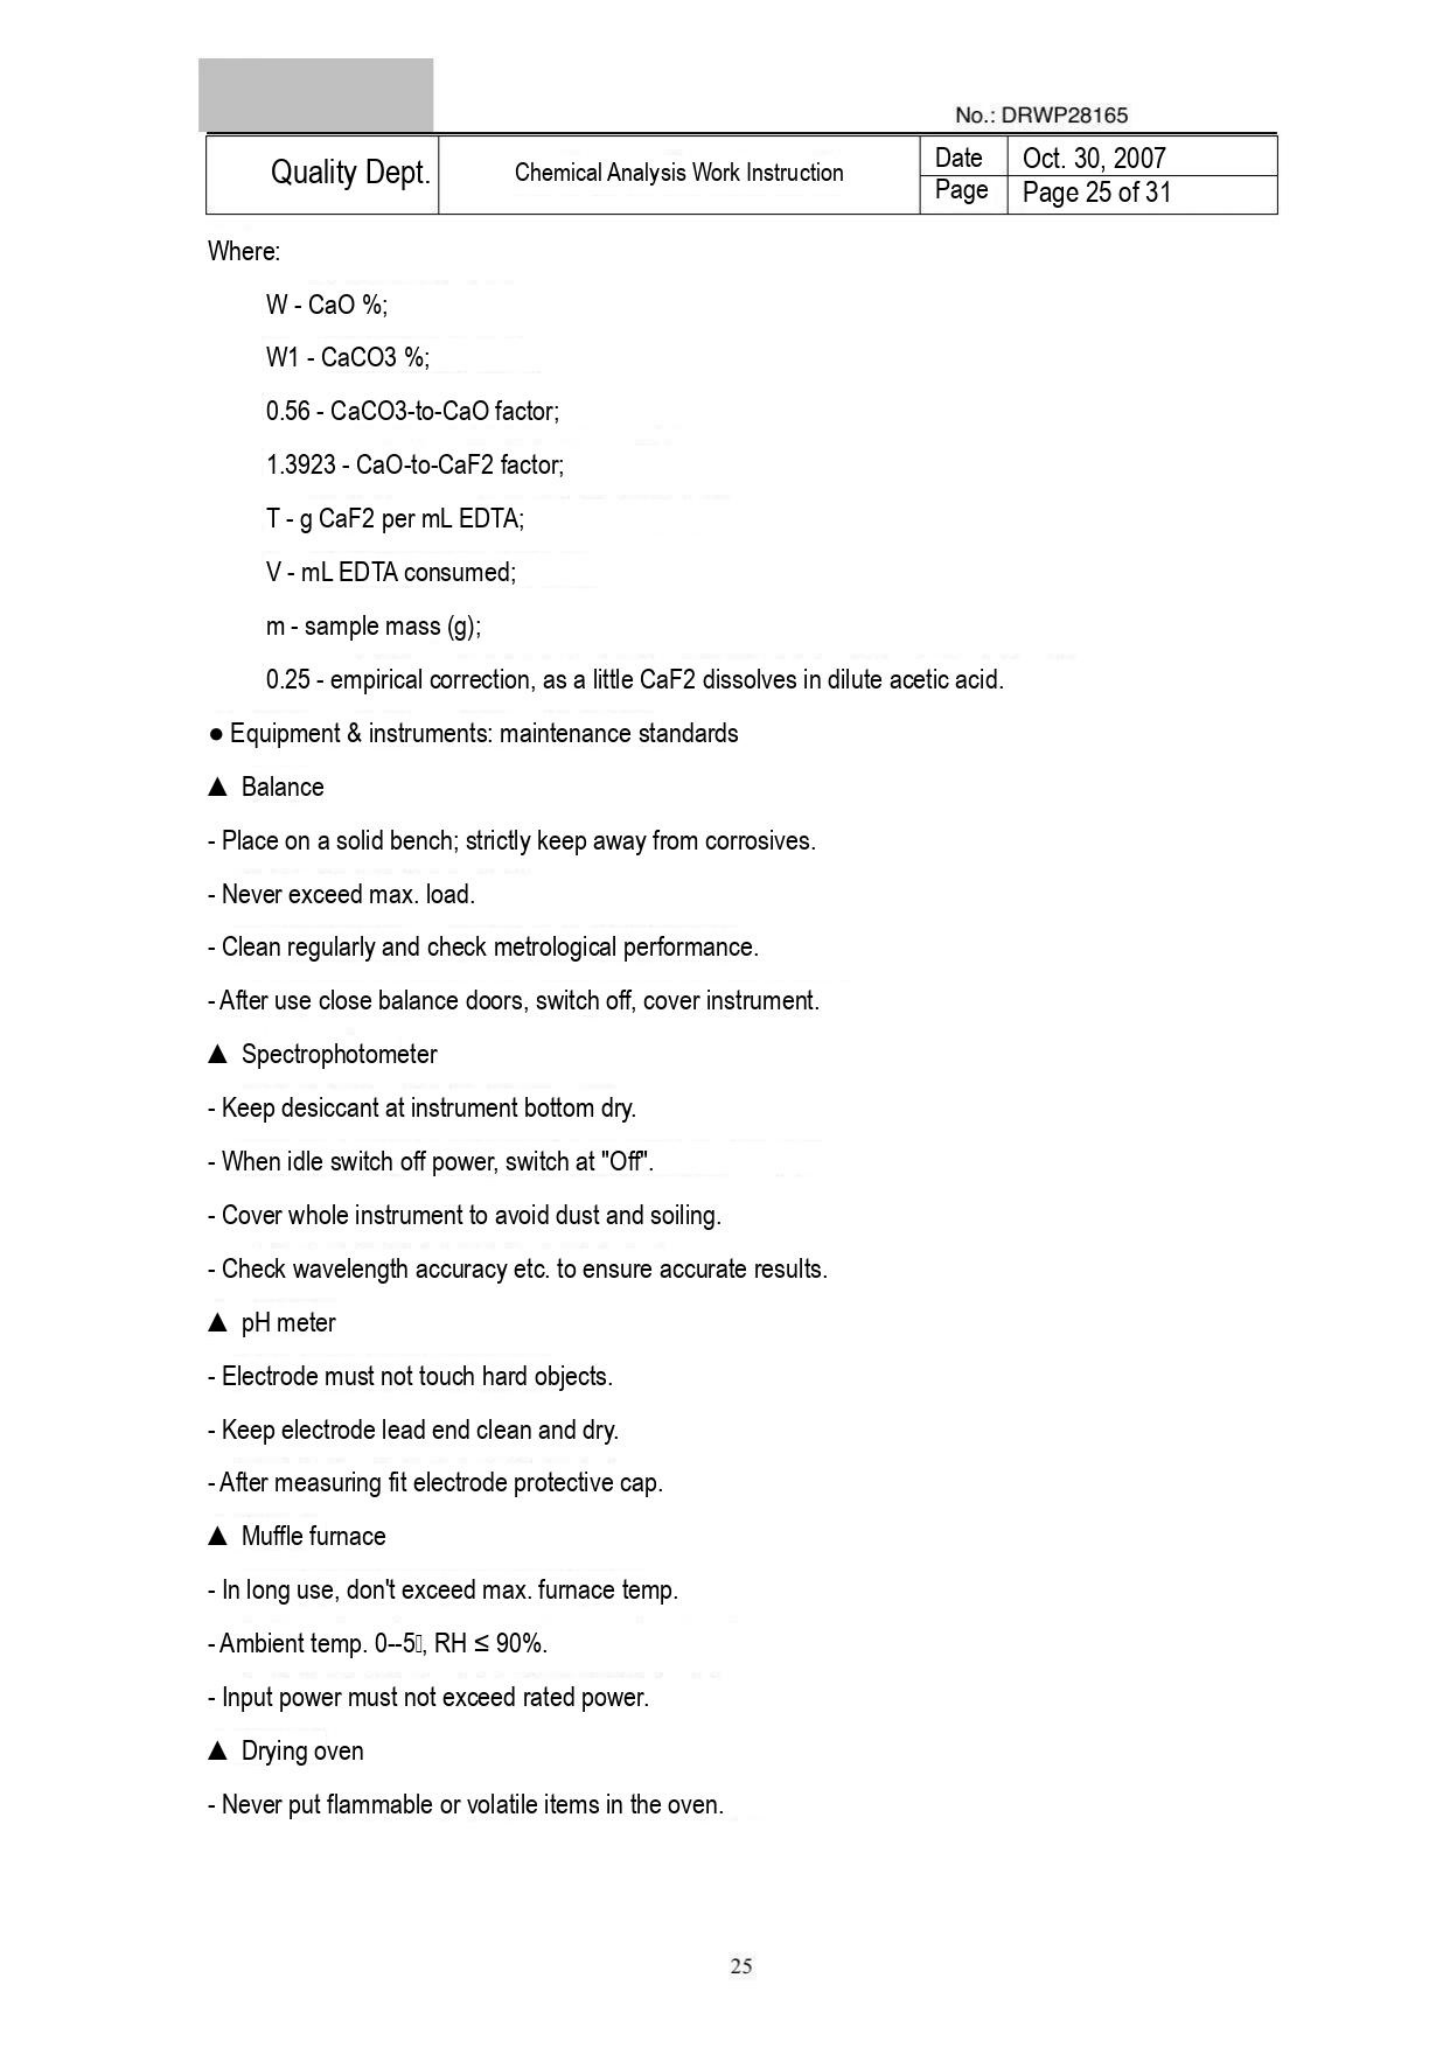No.: DRWP28165

| Quality Dept. | Chemical Analysis Work Instruction | Date | Oct. 30, 2007 |
|---|---|---|---|
| | | Page | Page 25 of 31 |

Where:

W - CaO %;

W1 - CaCO3 %;

0.56 - CaCO3-to-CaO factor;

1.3923 - CaO-to-CaF2 factor;

T - g CaF2 per mL EDTA;

V - mL EDTA consumed;

m - sample mass (g);

0.25 - empirical correction, as a little CaF2 dissolves in dilute acetic acid.

● Equipment & instruments: maintenance standards

▲ Balance

- Place on a solid bench; strictly keep away from corrosives.

- Never exceed max. load.

- Clean regularly and check metrological performance.

- After use close balance doors, switch off, cover instrument.

▲ Spectrophotometer

- Keep desiccant at instrument bottom dry.

- When idle switch off power, switch at "Off".

- Cover whole instrument to avoid dust and soiling.

- Check wavelength accuracy etc. to ensure accurate results.

▲ pH meter

- Electrode must not touch hard objects.

- Keep electrode lead end clean and dry.

- After measuring fit electrode protective cap.

▲ Muffle furnace

- In long use, don't exceed max. furnace temp.

- Ambient temp. 0--5, RH ≤ 90%.

- Input power must not exceed rated power.

▲ Drying oven

- Never put flammable or volatile items in the oven.

25
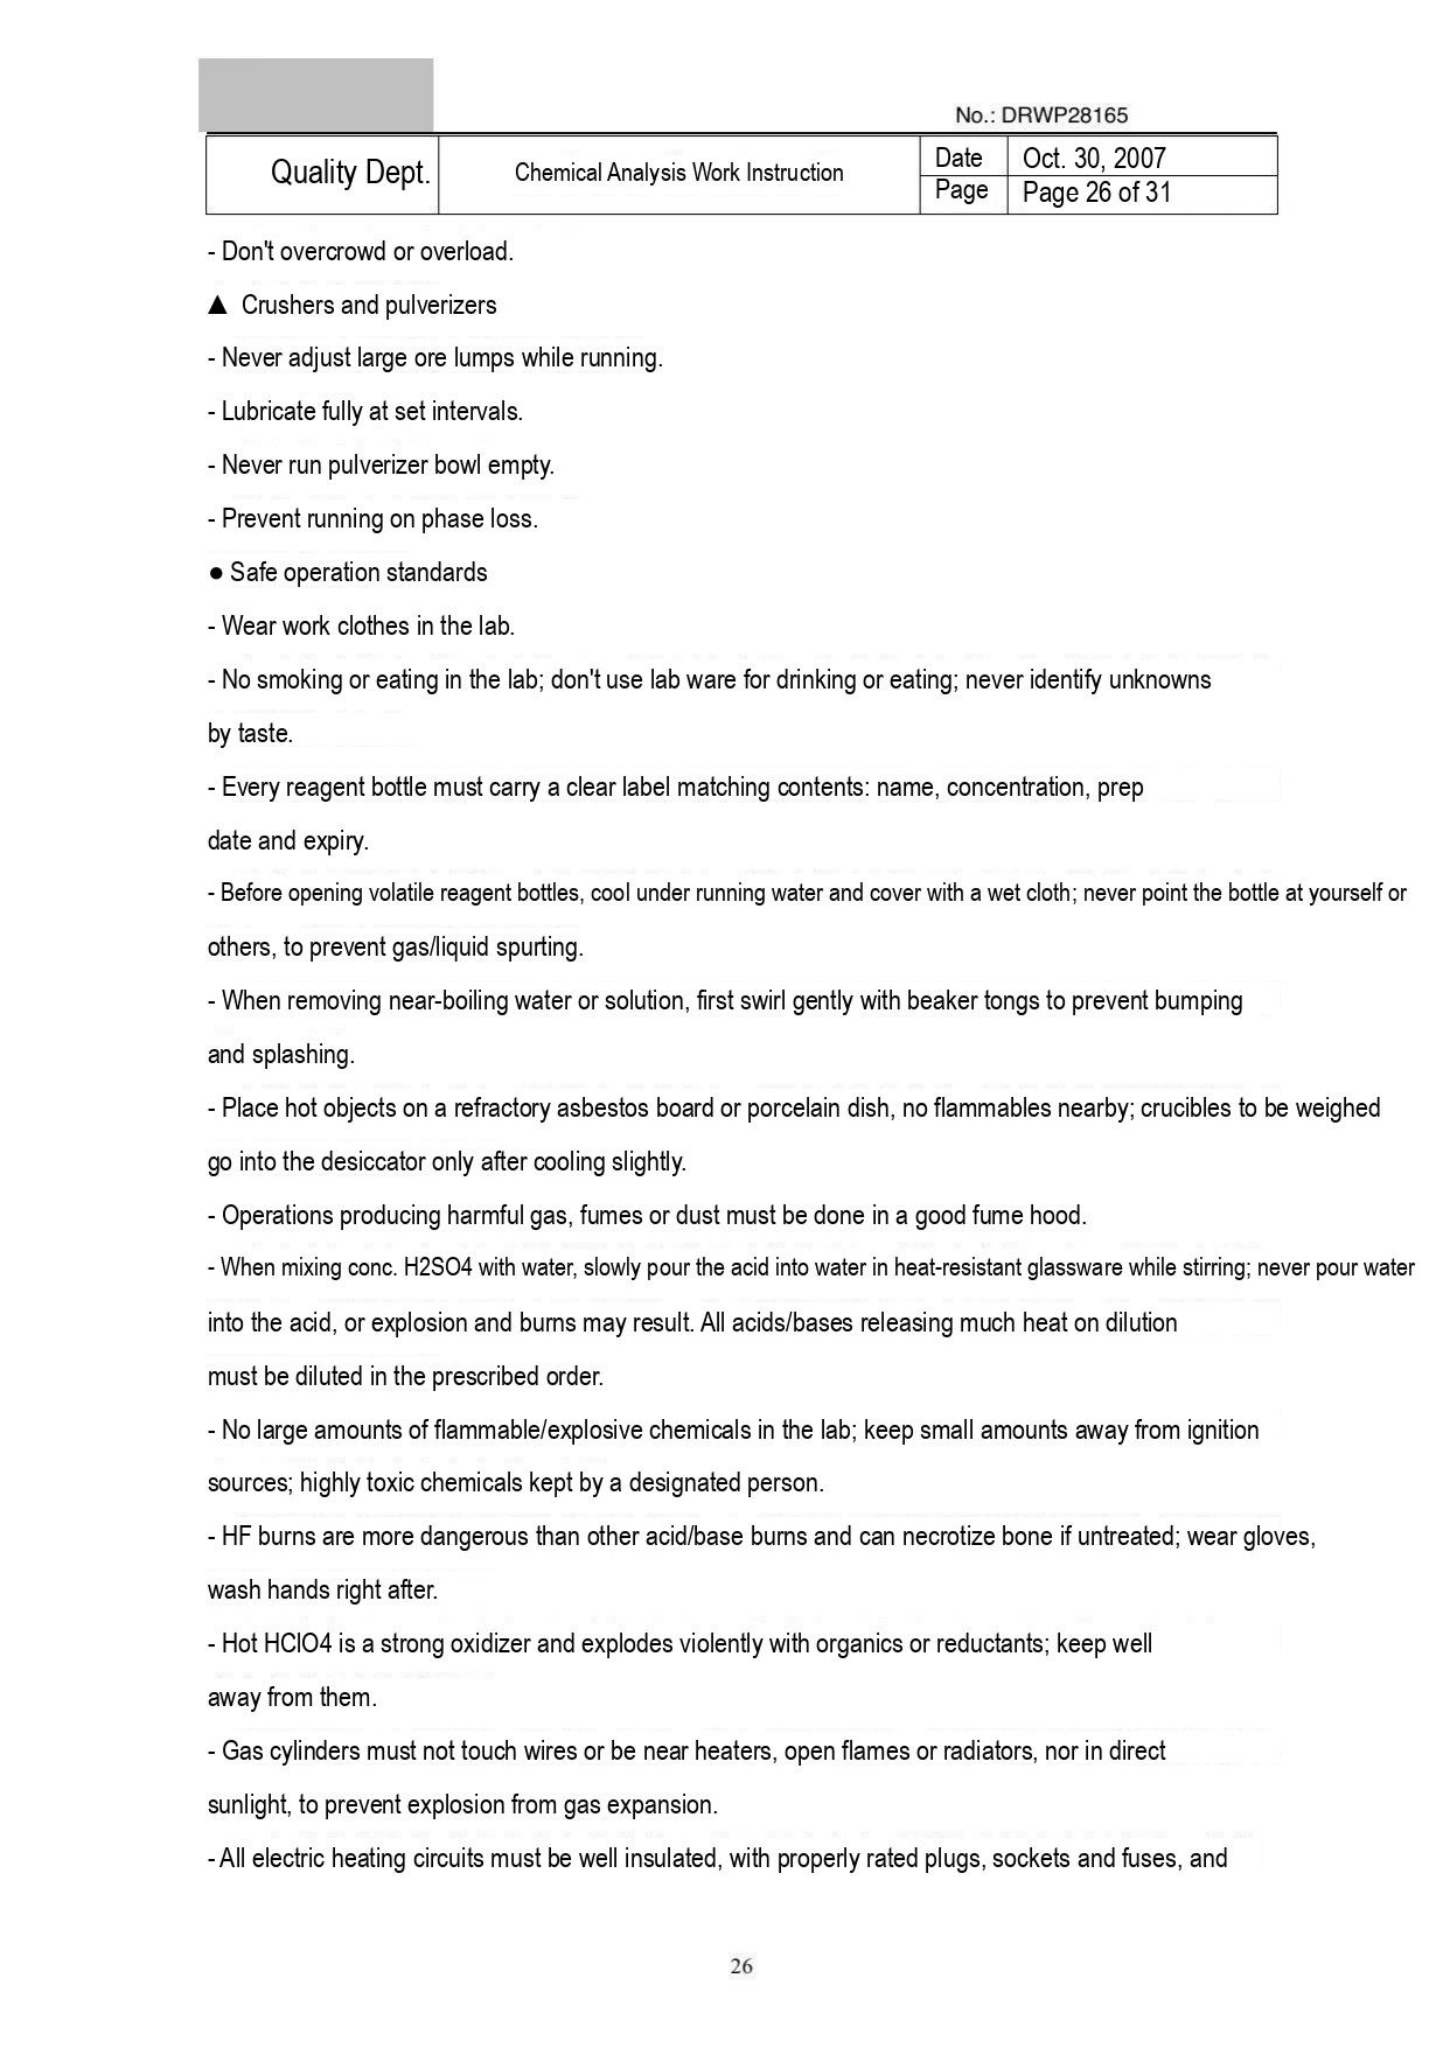No.: DRWP28165

| Quality Dept. | Chemical Analysis Work Instruction | Date | Oct. 30, 2007 |
|---|---|---|---|
| | | Page | Page 26 of 31 |

- Don't overcrowd or overload.

▲ Crushers and pulverizers

- Never adjust large ore lumps while running.

- Lubricate fully at set intervals.

- Never run pulverizer bowl empty.

- Prevent running on phase loss.

● Safe operation standards

- Wear work clothes in the lab.

- No smoking or eating in the lab; don't use lab ware for drinking or eating; never identify unknowns by taste.

- Every reagent bottle must carry a clear label matching contents: name, concentration, prep date and expiry.

- Before opening volatile reagent bottles, cool under running water and cover with a wet cloth; never point the bottle at yourself or others, to prevent gas/liquid spurting.

- When removing near-boiling water or solution, first swirl gently with beaker tongs to prevent bumping and splashing.

- Place hot objects on a refractory asbestos board or porcelain dish, no flammables nearby; crucibles to be weighed go into the desiccator only after cooling slightly.

- Operations producing harmful gas, fumes or dust must be done in a good fume hood.

- When mixing conc. H2SO4 with water, slowly pour the acid into water in heat-resistant glassware while stirring; never pour water into the acid, or explosion and burns may result. All acids/bases releasing much heat on dilution must be diluted in the prescribed order.

- No large amounts of flammable/explosive chemicals in the lab; keep small amounts away from ignition sources; highly toxic chemicals kept by a designated person.

- HF burns are more dangerous than other acid/base burns and can necrotize bone if untreated; wear gloves, wash hands right after.

- Hot HClO4 is a strong oxidizer and explodes violently with organics or reductants; keep well away from them.

- Gas cylinders must not touch wires or be near heaters, open flames or radiators, nor in direct sunlight, to prevent explosion from gas expansion.

- All electric heating circuits must be well insulated, with properly rated plugs, sockets and fuses, and

26
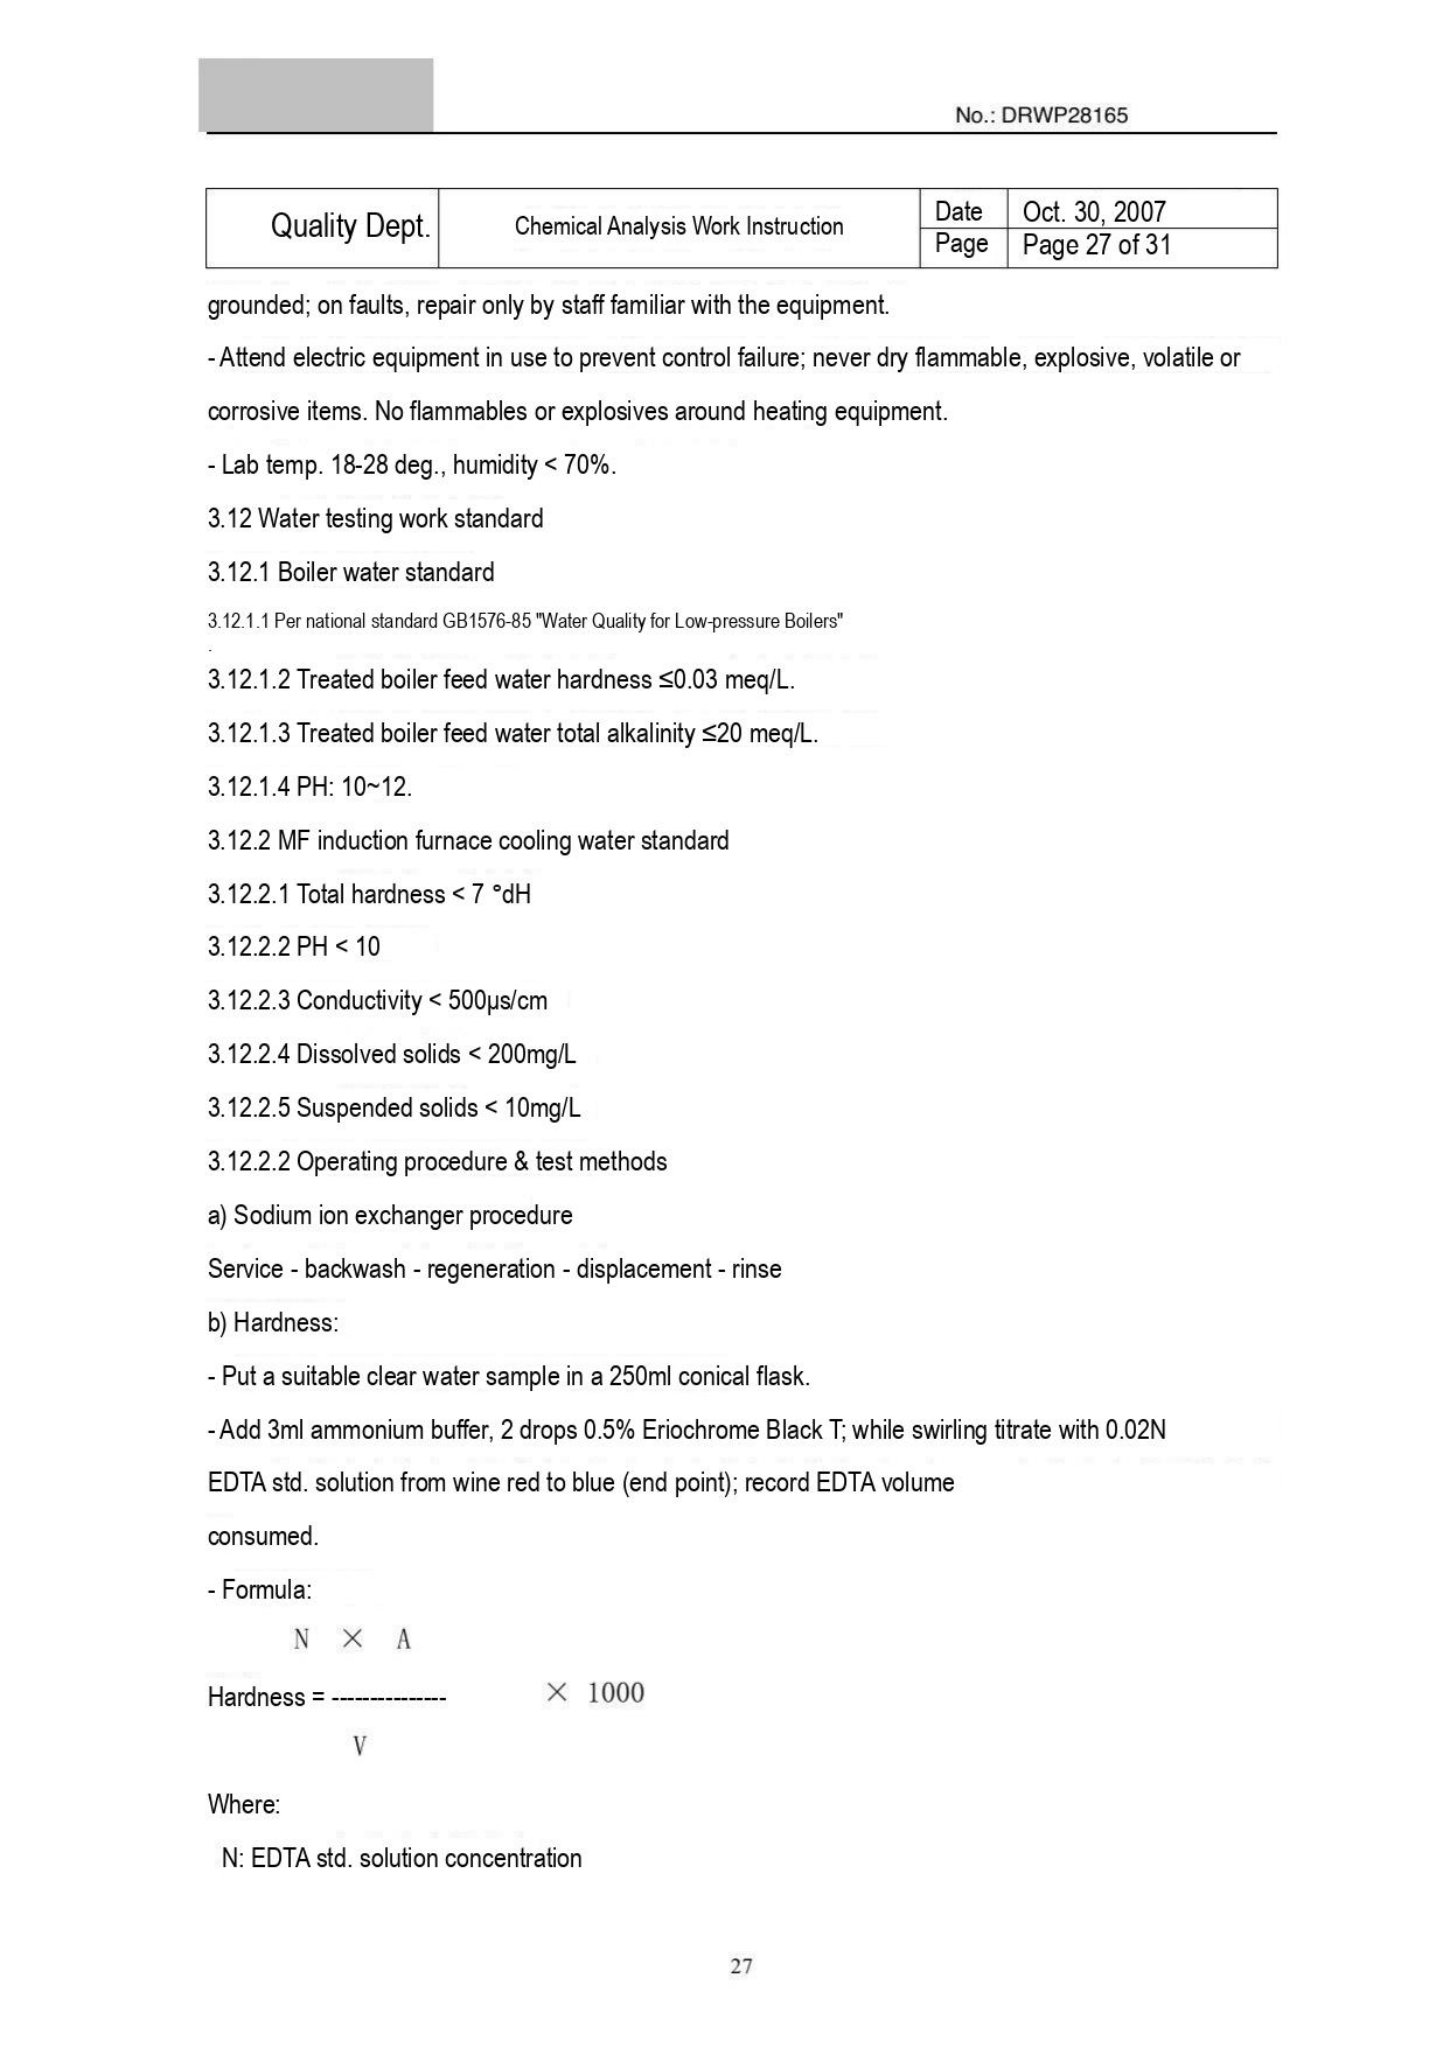No.: DRWP28165

| Quality Dept. | Chemical Analysis Work Instruction | Date | Oct. 30, 2007 |
|---|---|---|---|
| | | Page | Page 27 of 31 |

grounded; on faults, repair only by staff familiar with the equipment.

- Attend electric equipment in use to prevent control failure; never dry flammable, explosive, volatile or corrosive items. No flammables or explosives around heating equipment.

- Lab temp. 18-28 deg., humidity < 70%.

3.12 Water testing work standard

3.12.1 Boiler water standard

3.12.1.1 Per national standard GB1576-85 "Water Quality for Low-pressure Boilers"

3.12.1.2 Treated boiler feed water hardness ≤0.03 meq/L.

3.12.1.3 Treated boiler feed water total alkalinity ≤20 meq/L.

3.12.1.4 PH: 10~12.

3.12.2 MF induction furnace cooling water standard

3.12.2.1 Total hardness < 7 °dH

3.12.2.2 PH < 10

3.12.2.3 Conductivity < 500μs/cm

3.12.2.4 Dissolved solids < 200mg/L

3.12.2.5 Suspended solids < 10mg/L

3.12.2.2 Operating procedure & test methods

a) Sodium ion exchanger procedure

Service - backwash - regeneration - displacement - rinse

b) Hardness:

- Put a suitable clear water sample in a 250ml conical flask.

- Add 3ml ammonium buffer, 2 drops 0.5% Eriochrome Black T; while swirling titrate with 0.02N EDTA std. solution from wine red to blue (end point); record EDTA volume consumed.

- Formula:

N × A

Hardness = -------------- × 1000

V

Where:

N: EDTA std. solution concentration

27
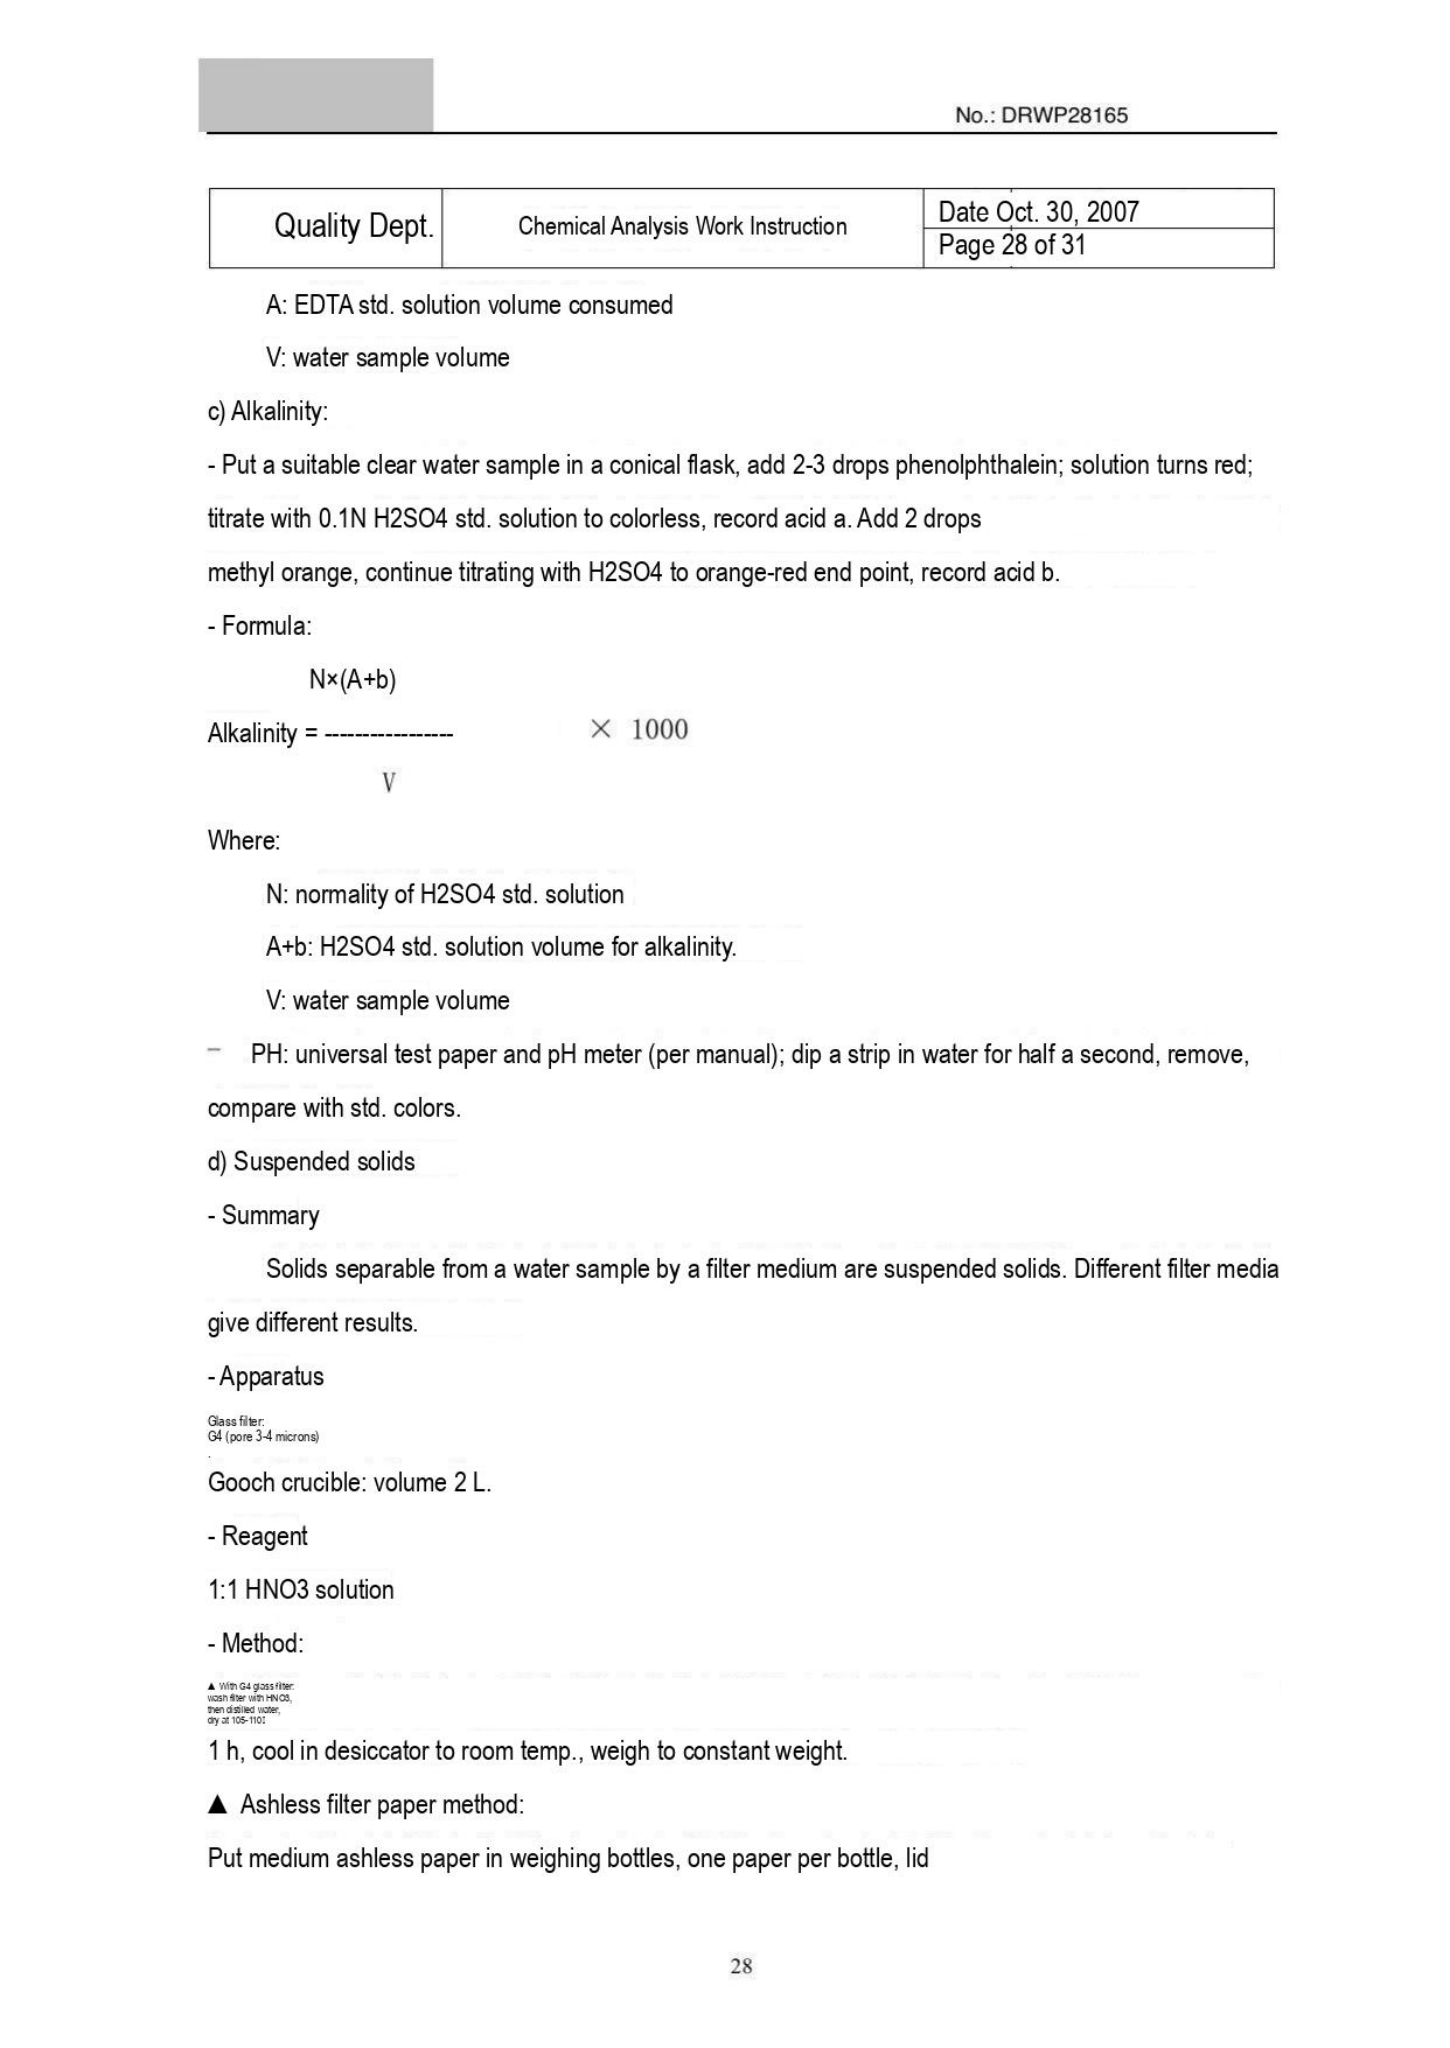No.: DRWP28165

| Quality Dept. | Chemical Analysis Work Instruction | Date Oct. 30, 2007<br>Page 28 of 31 |
|---|---|---|

A: EDTA std. solution volume consumed

V: water sample volume

c) Alkalinity:

- Put a suitable clear water sample in a conical flask, add 2-3 drops phenolphthalein; solution turns red; titrate with 0.1N H2SO4 std. solution to colorless, record acid a. Add 2 drops methyl orange, continue titrating with H2SO4 to orange-red end point, record acid b.

- Formula:

N×(A+b)

Alkalinity = ---------------- × 1000

V

Where:

N: normality of H2SO4 std. solution

A+b: H2SO4 std. solution volume for alkalinity.

V: water sample volume

– PH: universal test paper and pH meter (per manual); dip a strip in water for half a second, remove, compare with std. colors.

d) Suspended solids

- Summary

Solids separable from a water sample by a filter medium are suspended solids. Different filter media give different results.

- Apparatus

Glass filter:
G4 (pore 3-4 microns)

Gooch crucible: volume 2 L.

- Reagent

1:1 HNO3 solution

- Method:

▲ With G4 glass filter:
wash filter with HNO3,
then distilled water,
dry at 105-110

1 h, cool in desiccator to room temp., weigh to constant weight.

▲ Ashless filter paper method:

Put medium ashless paper in weighing bottles, one paper per bottle, lid

28
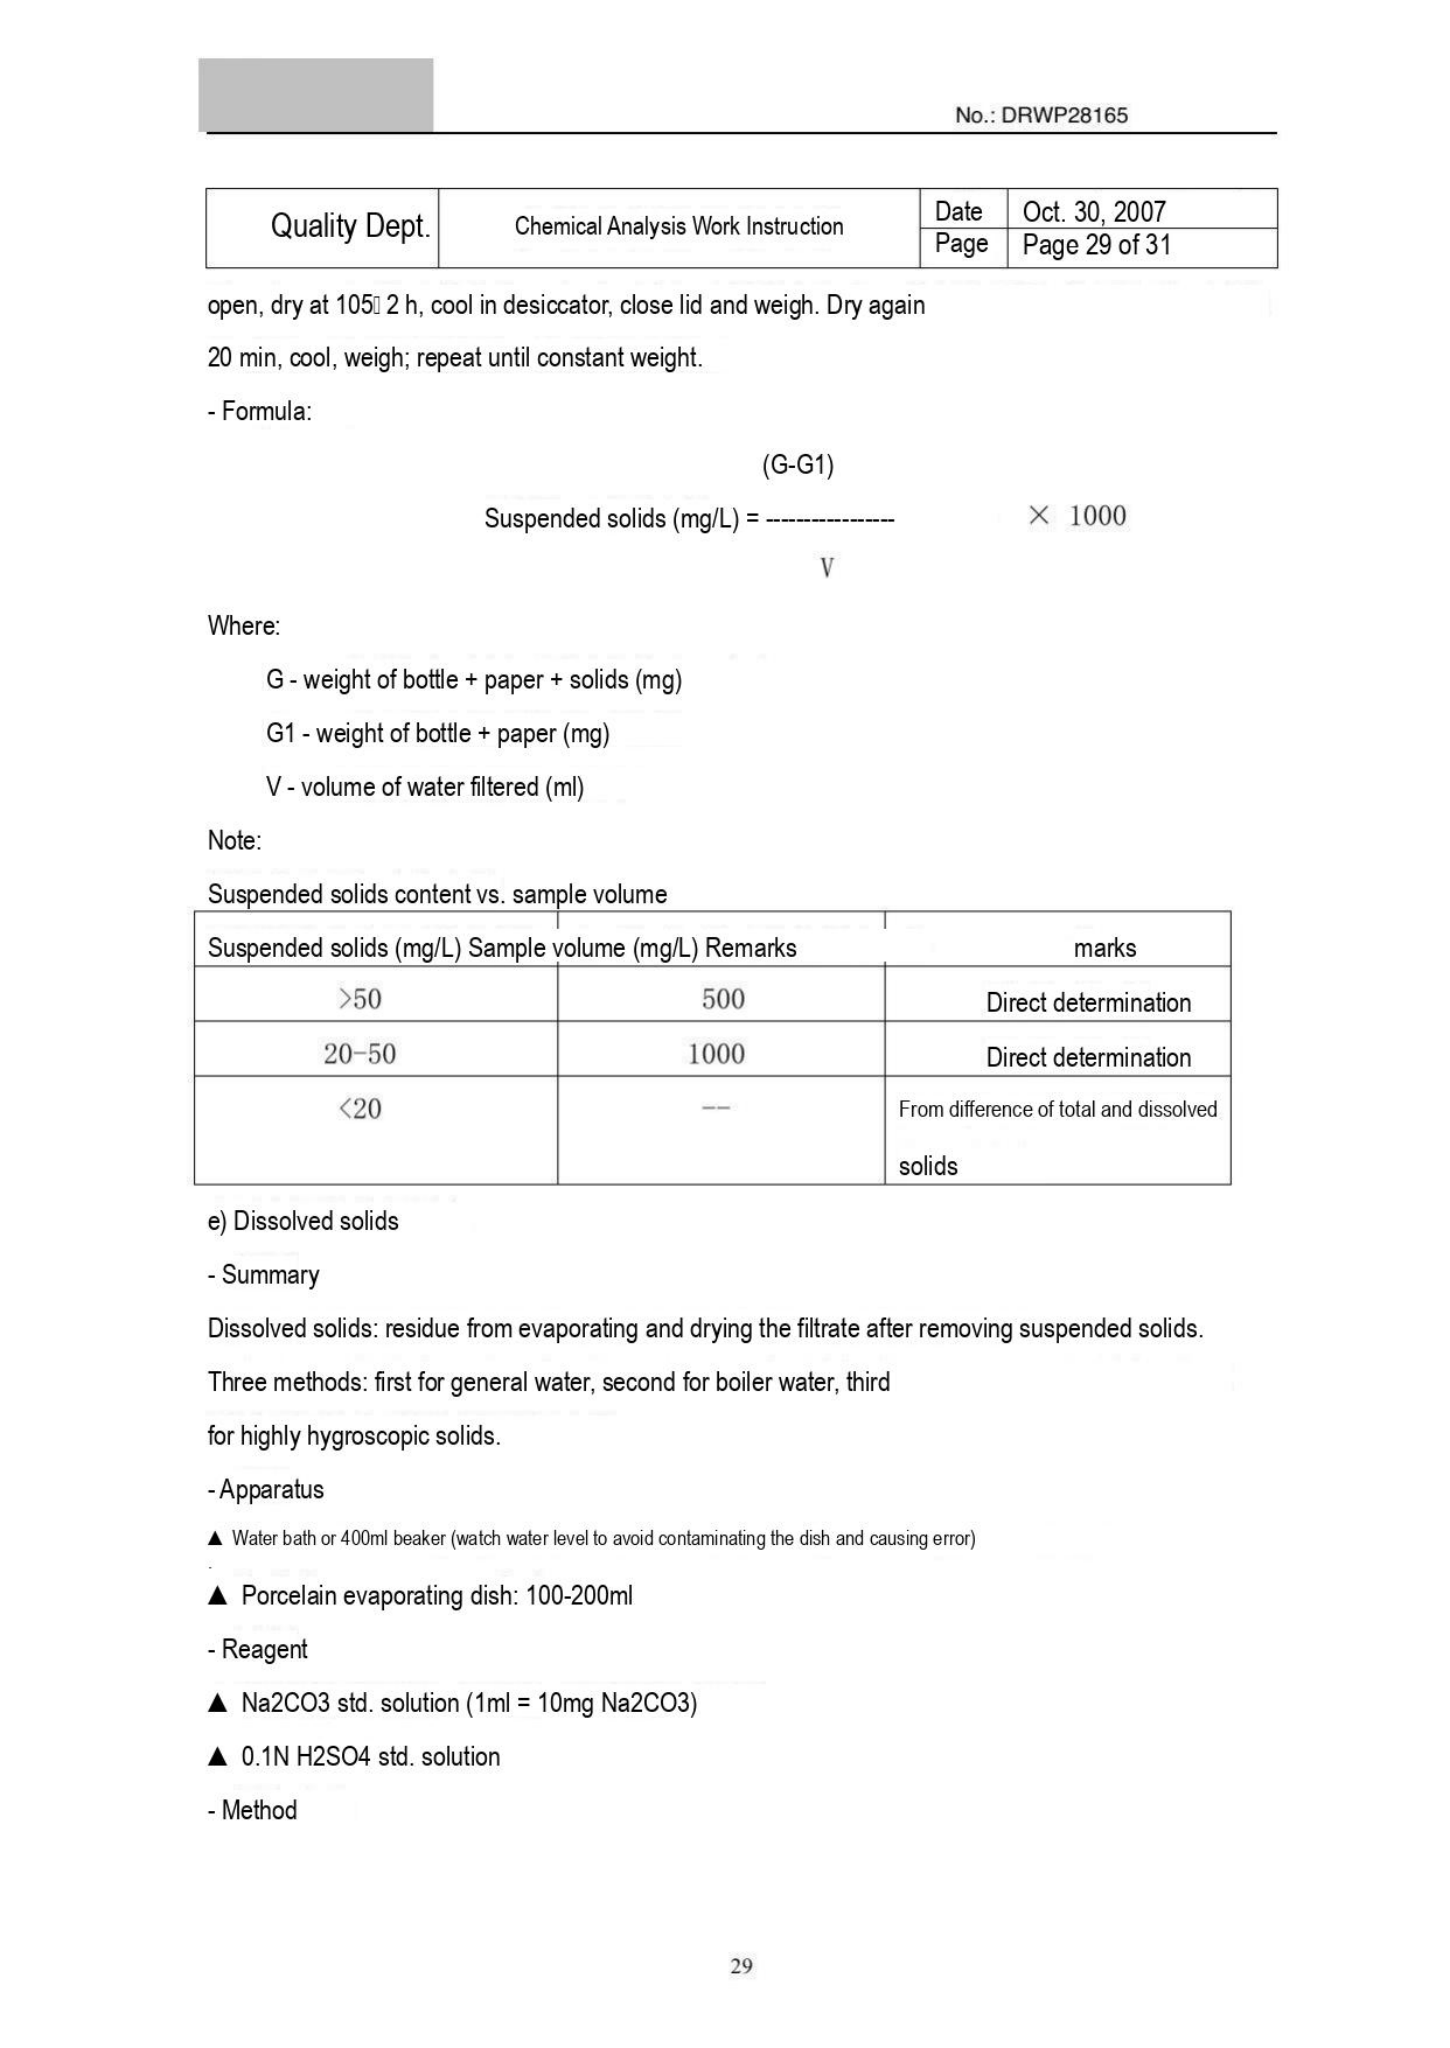No.: DRWP28165

| Quality Dept. | Chemical Analysis Work Instruction | Date | Oct. 30, 2007 |
|---|---|---|---|
| | | Page | Page 29 of 31 |

open, dry at 105 2 h, cool in desiccator, close lid and weigh. Dry again

20 min, cool, weigh; repeat until constant weight.

- Formula:

(G-G1)

Suspended solids (mg/L) = ---------------- × 1000

V

Where:

G - weight of bottle + paper + solids (mg)

G1 - weight of bottle + paper (mg)

V - volume of water filtered (ml)

Note:

Suspended solids content vs. sample volume

| Suspended solids (mg/L) Sample volume (mg/L) Remarks | | marks |
|---|---|---|
| >50 | 500 | Direct determination |
| 20−50 | 1000 | Direct determination |
| <20 | -- | From difference of total and dissolved solids |

e) Dissolved solids

- Summary

Dissolved solids: residue from evaporating and drying the filtrate after removing suspended solids.

Three methods: first for general water, second for boiler water, third

for highly hygroscopic solids.

- Apparatus

▲ Water bath or 400ml beaker (watch water level to avoid contaminating the dish and causing error)

▲ Porcelain evaporating dish: 100-200ml

- Reagent

▲ Na2CO3 std. solution (1ml = 10mg Na2CO3)

▲ 0.1N H2SO4 std. solution

- Method

29
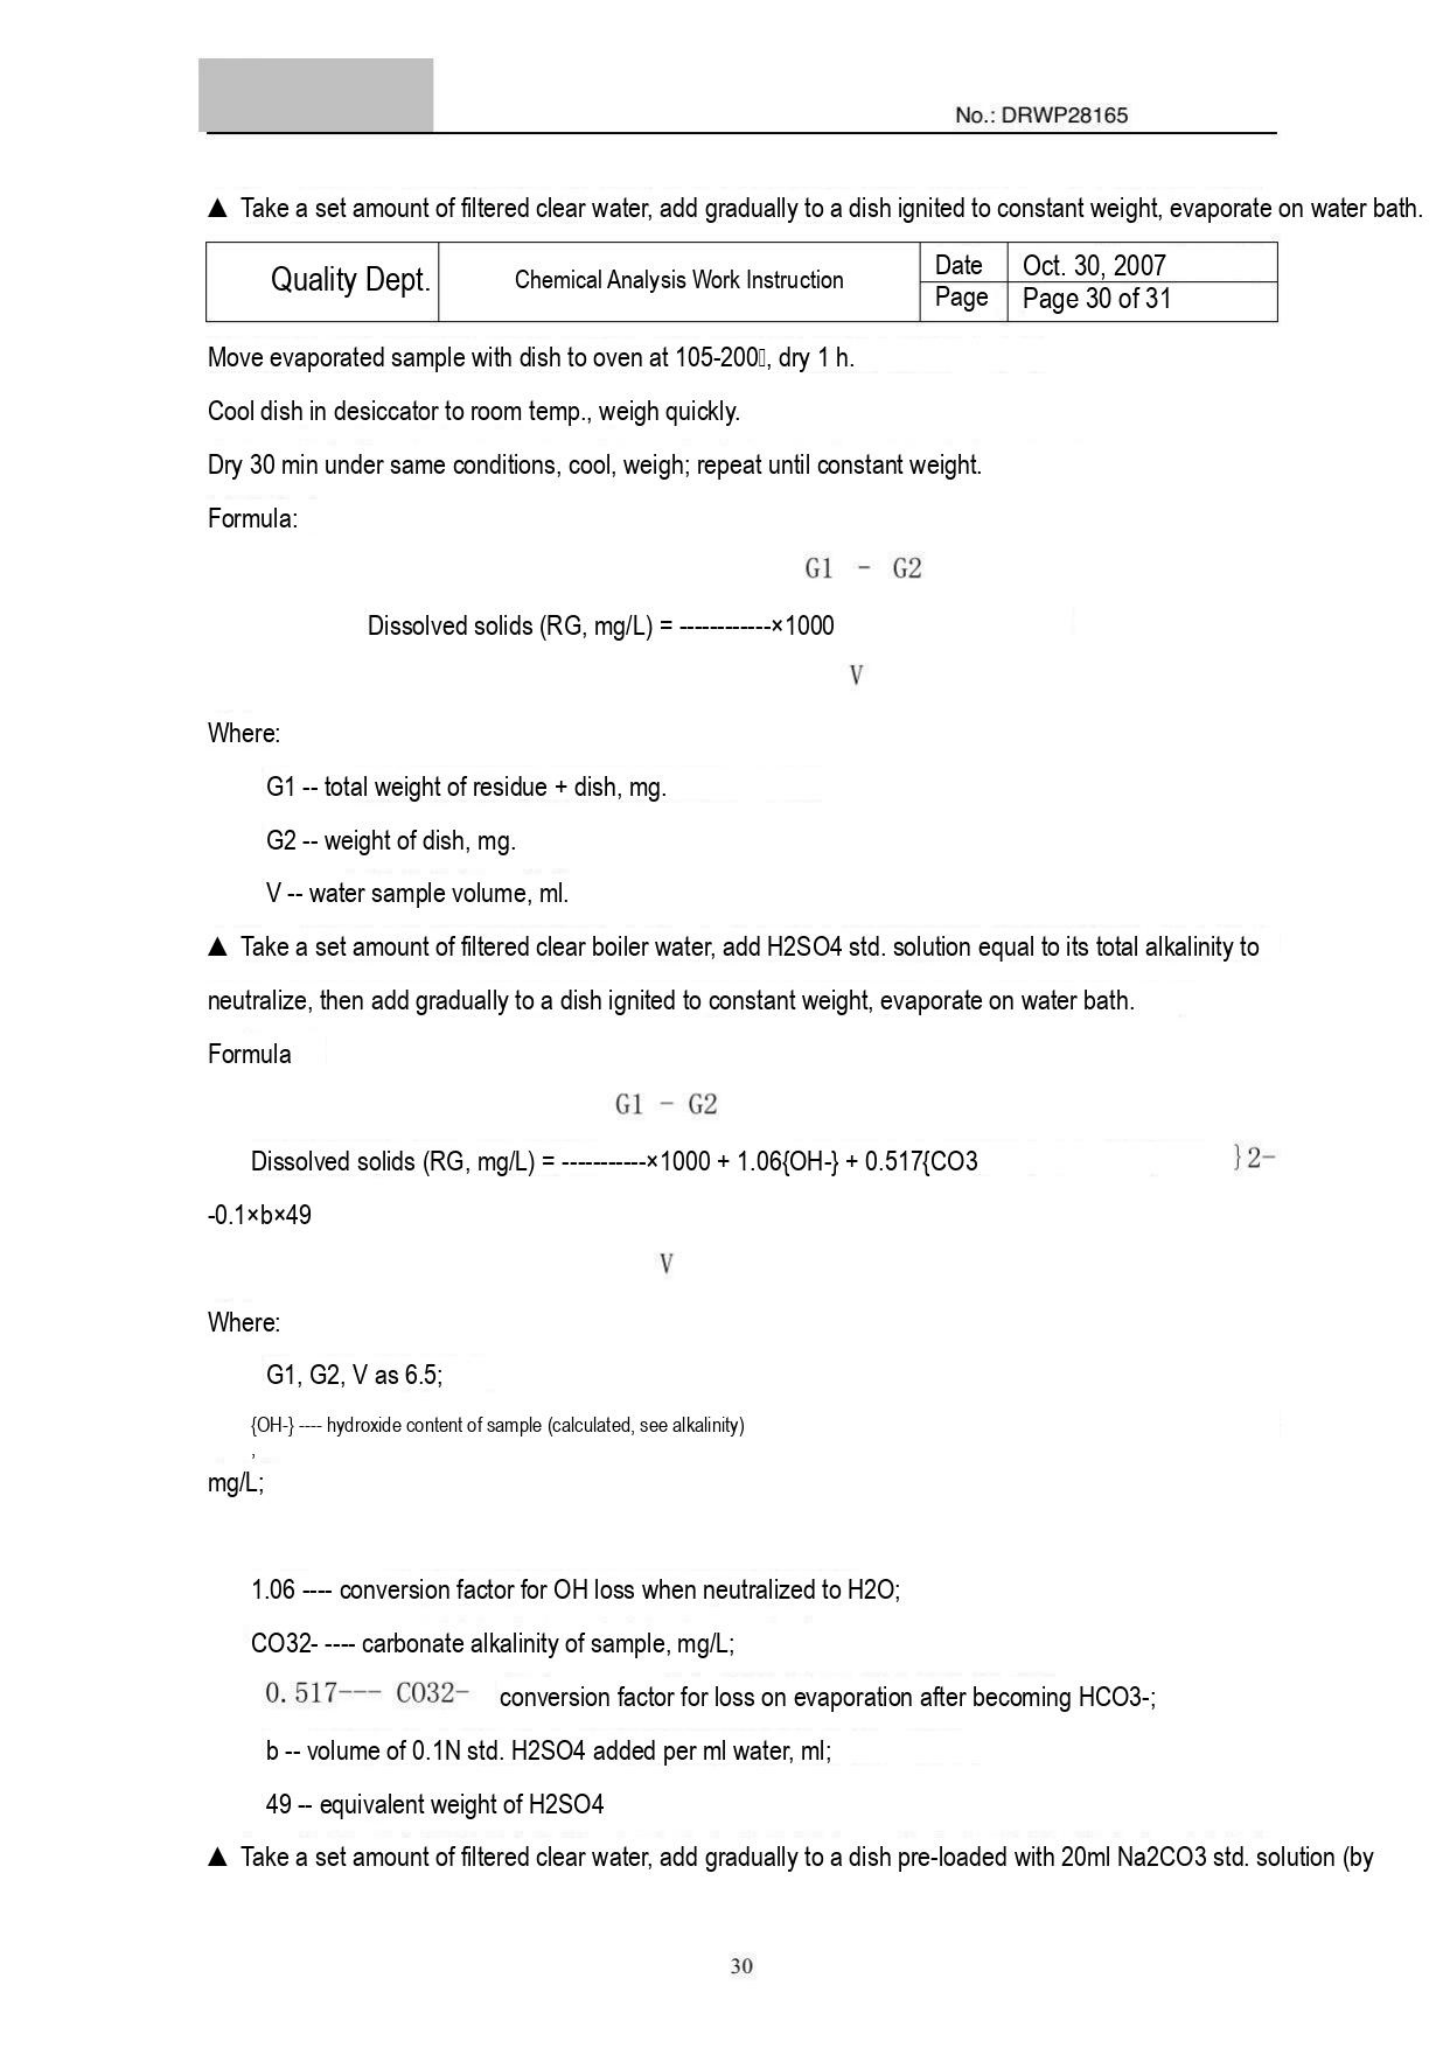No.: DRWP28165

▲ Take a set amount of filtered clear water, add gradually to a dish ignited to constant weight, evaporate on water bath.

| Quality Dept. | Chemical Analysis Work Instruction | Date | Oct. 30, 2007 |
|---|---|---|---|
| | | Page | Page 30 of 31 |

Move evaporated sample with dish to oven at 105-200, dry 1 h.

Cool dish in desiccator to room temp., weigh quickly.

Dry 30 min under same conditions, cool, weigh; repeat until constant weight.

Formula:

G1 - G2

Dissolved solids (RG, mg/L) = -----------×1000

V

Where:

G1 -- total weight of residue + dish, mg.

G2 -- weight of dish, mg.

V -- water sample volume, ml.

▲ Take a set amount of filtered clear boiler water, add H2SO4 std. solution equal to its total alkalinity to neutralize, then add gradually to a dish ignited to constant weight, evaporate on water bath.

Formula

G1 - G2

Dissolved solids (RG, mg/L) = ----------×1000 + 1.06{OH-} + 0.517{CO3 }2-

-0.1×b×49

V

Where:

G1, G2, V as 6.5;

{OH-} ---- hydroxide content of sample (calculated, see alkalinity)

,

mg/L;

1.06 ---- conversion factor for OH loss when neutralized to H2O;

CO32- ---- carbonate alkalinity of sample, mg/L;

0.517--- CO32- conversion factor for loss on evaporation after becoming HCO3-;

b -- volume of 0.1N std. H2SO4 added per ml water, ml;

49 -- equivalent weight of H2SO4

▲ Take a set amount of filtered clear water, add gradually to a dish pre-loaded with 20ml Na2CO3 std. solution (by

30
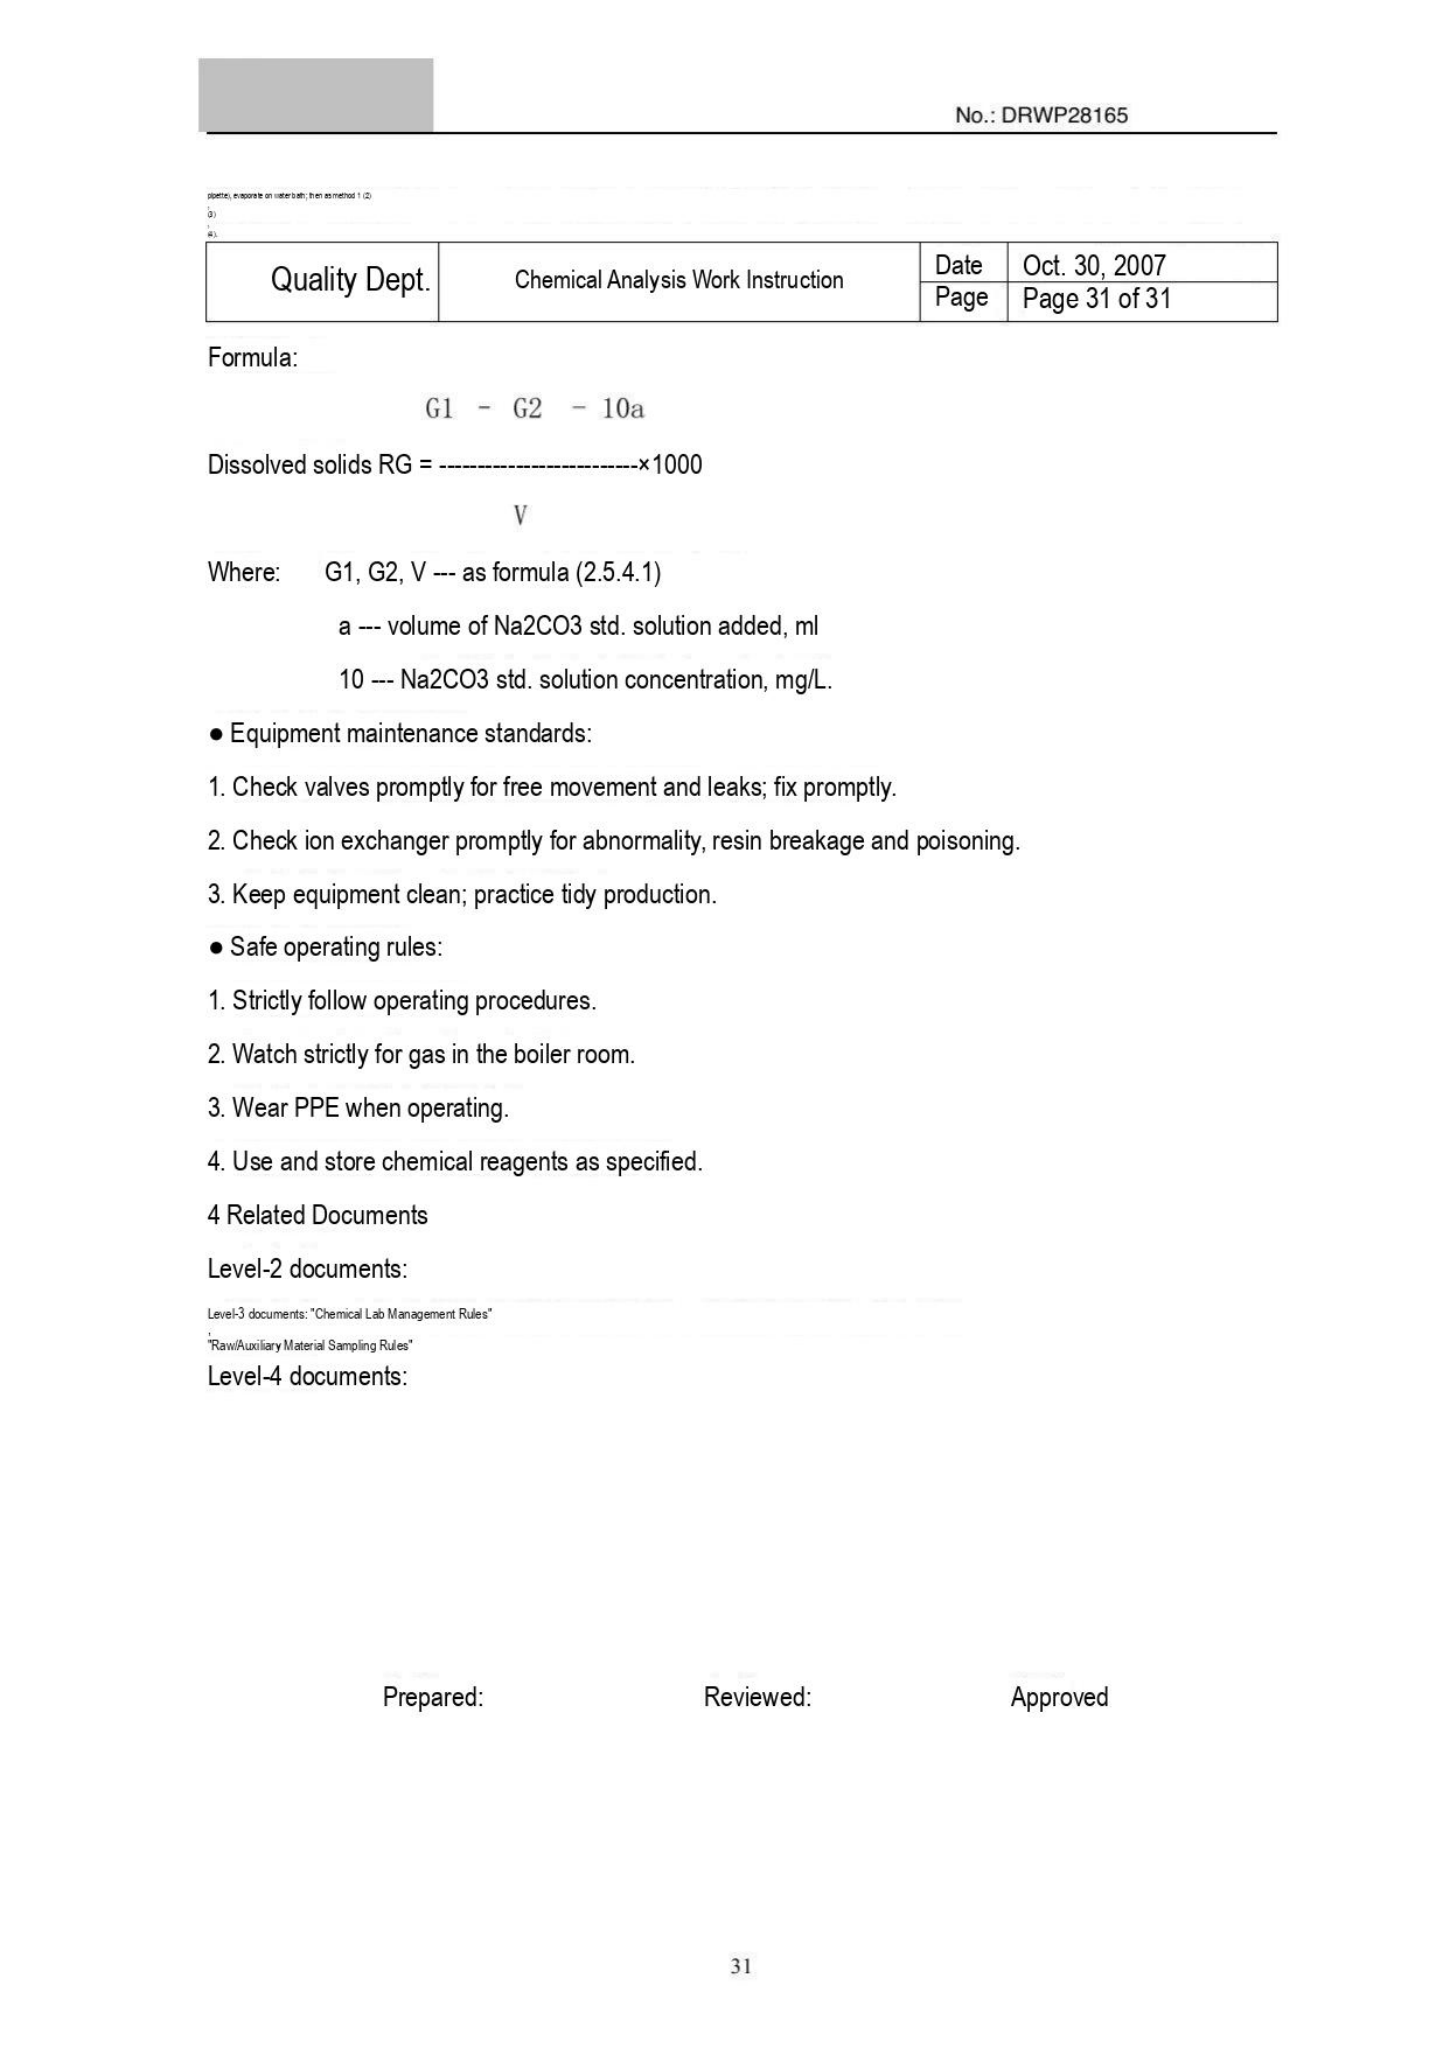No.: DRWP28165

pipette), evaporate on water bath; then as method 1 (2)

3)

4).

| Quality Dept. | Chemical Analysis Work Instruction | Date | Oct. 30, 2007 |
|---|---|---|---|
| | | Page | Page 31 of 31 |

Formula:

G1 - G2 - 10a

Dissolved solids RG = ------------------------×1000

V

Where: G1, G2, V --- as formula (2.5.4.1)

a --- volume of Na2CO3 std. solution added, ml

10 --- Na2CO3 std. solution concentration, mg/L.

● Equipment maintenance standards:

1. Check valves promptly for free movement and leaks; fix promptly.

2. Check ion exchanger promptly for abnormality, resin breakage and poisoning.

3. Keep equipment clean; practice tidy production.

● Safe operating rules:

1. Strictly follow operating procedures.

2. Watch strictly for gas in the boiler room.

3. Wear PPE when operating.

4. Use and store chemical reagents as specified.

4 Related Documents

Level-2 documents:

Level-3 documents: "Chemical Lab Management Rules"

"Raw/Auxiliary Material Sampling Rules"

Level-4 documents:

Prepared: Reviewed: Approved

31